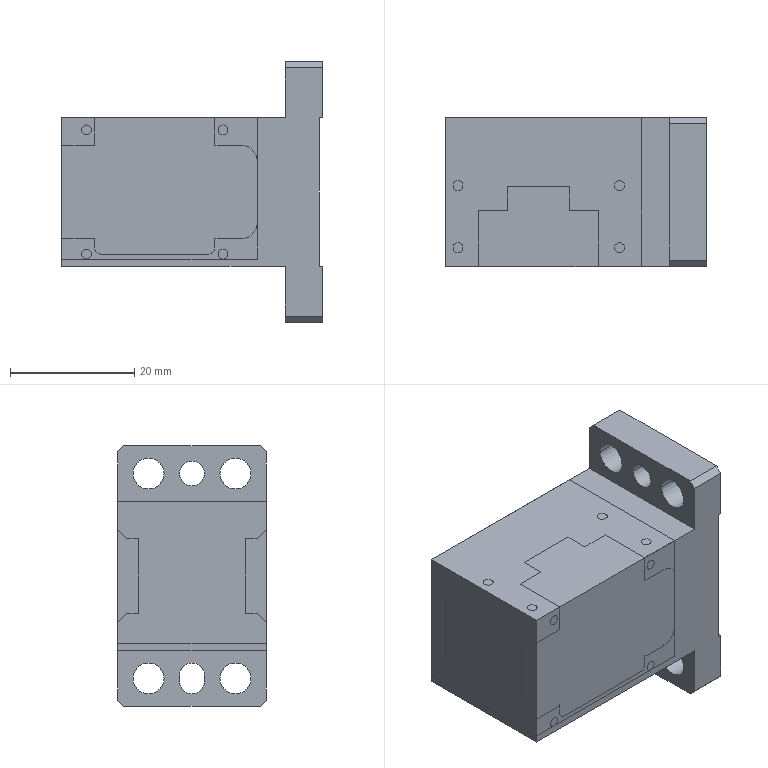NC program | NX | posted with a generic post | part box 42 x 24 x 42 mm
Lines 93 to 952 of 10692:
(ZLEVEL_PROFILE_1 , TOOL : D3)
N172 T03 M6
N174 G54
N176 G17 G0 G90 X-0.064 Y16.054 B0. C0. S6000 M3
N178 G43 Z30. H3
N180 Z0.8
N182 G94 G1 X0.019 Y16.04 Z0.796 F1000.
N184 X0.199 Y16.085 Z0.786
N186 X0.347 Y16.198 Z0.776
N188 X0.44 Y16.364 Z0.766
N190 X0.45 Y16.406 Z0.764
N192 Y16.596 Z0.754
N194 X0.417 Y16.693 Z0.749
N196 X0.303 Y16.846 Z0.739
N198 X0.095 Y16.95 Z0.726
N200 X-0.095 Z0.716
N202 X-0.303 Y16.846 Z0.704
N204 X-0.417 Y16.693 Z0.694
N206 X-0.45 Y16.596 Z0.689
N208 Y16.405 Z0.679
N210 X-0.324 Y16.174 Z0.665
N212 X-0.164 Y16.07 Z0.655
N214 X0.019 Y16.04 Z0.645
N216 X0.199 Y16.085 Z0.636
N218 X0.347 Y16.198 Z0.626
N220 X0.44 Y16.364 Z0.616
N222 X0.45 Y16.406 Z0.614
N224 Y16.596 Z0.604
N226 X0.417 Y16.693 Z0.598
N228 X0.303 Y16.846 Z0.588
N230 X0.095 Y16.95 Z0.576
N232 X-0.095 Z0.566
N234 X-0.303 Y16.846 Z0.554
N236 X-0.417 Y16.693 Z0.544
N238 X-0.45 Y16.596 Z0.539
N240 Y16.405 Z0.529
N242 X-0.324 Y16.174 Z0.515
N244 X-0.164 Y16.07 Z0.505
N246 X0.019 Y16.04 Z0.495
N248 X0.199 Y16.085 Z0.485
N250 X0.347 Y16.198 Z0.476
N252 X0.44 Y16.364 Z0.466
N254 X0.45 Y16.406 Z0.463
N256 Y16.596 Z0.453
N258 X0.417 Y16.693 Z0.448
N260 X0.303 Y16.846 Z0.438
N262 X0.095 Y16.95 Z0.426
N264 X-0.095 Z0.416
N266 X-0.303 Y16.846 Z0.404
N268 X-0.417 Y16.693 Z0.394
N270 X-0.45 Y16.596 Z0.388
N272 Y16.405 Z0.378
N274 X-0.324 Y16.174 Z0.364
N276 X-0.164 Y16.07 Z0.354
N278 X0.019 Y16.04 Z0.345
N280 X0.199 Y16.085 Z0.335
N282 X0.347 Y16.198 Z0.325
N284 X0.44 Y16.364 Z0.315
N286 X0.45 Y16.406 Z0.313
N288 Y16.596 Z0.303
N290 X0.417 Y16.693 Z0.298
N292 X0.303 Y16.846 Z0.288
N294 X0.095 Y16.95 Z0.276
N296 X-0.095 Z0.266
N298 X-0.303 Y16.846 Z0.253
N300 X-0.417 Y16.693 Z0.243
N302 X-0.45 Y16.596 Z0.238
N304 Y16.405 Z0.228
N306 X-0.324 Y16.174 Z0.214
N308 X-0.164 Y16.07 Z0.204
N310 X0.019 Y16.04 Z0.194
N312 X0.199 Y16.085 Z0.185
N314 X0.347 Y16.198 Z0.175
N316 X0.44 Y16.364 Z0.165
N318 X0.45 Y16.406 Z0.163
N320 Y16.596 Z0.153
N322 X0.417 Y16.693 Z0.147
N324 X0.303 Y16.846 Z0.137
N326 X0.095 Y16.95 Z0.125
N328 X-0.095 Z0.115
N330 X-0.303 Y16.846 Z0.103
N332 X-0.417 Y16.693 Z0.093
N334 X-0.45 Y16.596 Z0.088
N336 Y16.405 Z0.078
N338 X-0.324 Y16.174 Z0.064
N340 X-0.164 Y16.07 Z0.054
N342 X0.019 Y16.04 Z0.044
N344 X0.199 Y16.085 Z0.034
N346 X0.347 Y16.198 Z0.025
N348 X0.44 Y16.364 Z0.015
N350 X0.45 Y16.406 Z0.013
N352 Y16.596 Z0.003
N354 X0.417 Y16.693 Z-0.003
N356 X0.303 Y16.846 Z-0.013
N358 X0.095 Y16.95 Z-0.025
N360 X0. Z-0.03
N362 G3 X-0.45 Y16.5 R0.45
N364 X0. Y16.95 R-0.45
N366 G1 X-0.124 Y16.924 Z-0.032
N368 X-0.202 Y16.891 Z-0.034
N370 X-0.274 Y16.845 Z-0.035
N372 X-0.308 Y16.819 Z-0.036
N374 X-0.361 Y16.756 Z-0.038
N376 X-0.403 Y16.681 Z-0.039
N378 X-0.418 Y16.643 Z-0.04
N380 X-0.427 Y16.616
N382 X-0.438 Y16.561 Z-0.041
N384 X-0.441 Y16.475 Z-0.043
N386 X-0.437 Y16.433 Z-0.044
N388 X-0.432 Y16.406
N390 X-0.417 Y16.353 Z-0.045
N392 X-0.38 Y16.275 Z-0.047
N394 X-0.357 Y16.24
N396 X-0.341 Y16.218 Z-0.048
N398 X-0.303 Y16.178 Z-0.049
N400 X-0.234 Y16.126 Z-0.05
N402 X-0.198 Y16.105 Z-0.051
N404 X-0.173 Y16.093 Z-0.052
N406 X-0.121 Y16.075 Z-0.053
N408 X-0.039 Y16.06 Z-0.054
N410 X0.002 Y16.056 Z-0.055
N412 X0.088 Y16.066 Z-0.056
N414 X0.188 Y16.101 Z-0.058
N416 X0.282 Y16.149 Z-0.06
N418 G3 X0. Y16.95 R0.45
N420 G1 X-0.124 Y16.924 Z-0.062
N422 X-0.202 Y16.891 Z-0.064
N424 X-0.274 Y16.845 Z-0.065
N426 X-0.308 Y16.819 Z-0.066
N428 X-0.361 Y16.756 Z-0.068
N430 X-0.403 Y16.681 Z-0.069
N432 X-0.418 Y16.643 Z-0.07
N434 X-0.427 Y16.616
N436 X-0.438 Y16.561 Z-0.071
N438 X-0.441 Y16.475 Z-0.073
N440 X-0.437 Y16.433 Z-0.074
N442 X-0.432 Y16.406
N444 X-0.417 Y16.353 Z-0.075
N446 X-0.38 Y16.275 Z-0.077
N448 X-0.357 Y16.24
N450 X-0.341 Y16.218 Z-0.078
N452 X-0.303 Y16.178 Z-0.079
N454 X-0.234 Y16.126 Z-0.08
N456 X-0.198 Y16.105 Z-0.081
N458 X-0.173 Y16.093 Z-0.082
N460 X-0.121 Y16.075 Z-0.083
N462 X-0.039 Y16.06 Z-0.084
N464 X0.002 Y16.056 Z-0.085
N466 X0.088 Y16.066 Z-0.086
N468 X0.188 Y16.101 Z-0.088
N470 X0.282 Y16.149 Z-0.09
N472 G3 X0. Y16.95 R0.45
N474 G1 X-0.124 Y16.924 Z-0.092
N476 X-0.202 Y16.891 Z-0.094
N478 X-0.274 Y16.845 Z-0.095
N480 X-0.308 Y16.819 Z-0.096
N482 X-0.361 Y16.756 Z-0.098
N484 X-0.403 Y16.681 Z-0.099
N486 X-0.418 Y16.643 Z-0.1
N488 X-0.427 Y16.616
N490 X-0.438 Y16.561 Z-0.101
N492 X-0.441 Y16.475 Z-0.103
N494 X-0.437 Y16.433 Z-0.104
N496 X-0.432 Y16.406
N498 X-0.417 Y16.353 Z-0.105
N500 X-0.38 Y16.275 Z-0.107
N502 X-0.357 Y16.24
N504 X-0.341 Y16.218 Z-0.108
N506 X-0.303 Y16.178 Z-0.109
N508 X-0.234 Y16.126 Z-0.11
N510 X-0.198 Y16.105 Z-0.111
N512 X-0.173 Y16.093 Z-0.112
N514 X-0.121 Y16.075 Z-0.113
N516 X-0.039 Y16.06 Z-0.114
N518 X0.002 Y16.056 Z-0.115
N520 X0.088 Y16.066 Z-0.116
N522 X0.188 Y16.101 Z-0.118
N524 X0.282 Y16.149 Z-0.12
N526 G3 X0. Y16.95 R0.45
N528 G1 X-0.124 Y16.924 Z-0.122
N530 X-0.202 Y16.891 Z-0.124
N532 X-0.274 Y16.845 Z-0.125
N534 X-0.308 Y16.819 Z-0.126
N536 X-0.361 Y16.756 Z-0.128
N538 X-0.403 Y16.681 Z-0.129
N540 X-0.418 Y16.643 Z-0.13
N542 X-0.427 Y16.616
N544 X-0.438 Y16.561 Z-0.131
N546 X-0.441 Y16.475 Z-0.133
N548 X-0.437 Y16.433 Z-0.134
N550 X-0.432 Y16.406
N552 X-0.417 Y16.353 Z-0.135
N554 X-0.38 Y16.275 Z-0.137
N556 X-0.357 Y16.24
N558 X-0.341 Y16.218 Z-0.138
N560 X-0.303 Y16.178 Z-0.139
N562 X-0.234 Y16.126 Z-0.14
N564 X-0.198 Y16.105 Z-0.141
N566 X-0.173 Y16.093 Z-0.142
N568 X-0.121 Y16.075 Z-0.143
N570 X-0.039 Y16.06 Z-0.144
N572 X0.002 Y16.056 Z-0.145
N574 X0.088 Y16.066 Z-0.146
N576 X0.188 Y16.101 Z-0.148
N578 X0.282 Y16.149 Z-0.15
N580 G3 X0. Y16.95 R0.45
N582 G1 X-0.124 Y16.924 Z-0.152
N584 X-0.202 Y16.891 Z-0.154
N586 X-0.274 Y16.845 Z-0.155
N588 X-0.308 Y16.819 Z-0.156
N590 X-0.361 Y16.756 Z-0.158
N592 X-0.403 Y16.681 Z-0.159
N594 X-0.418 Y16.643 Z-0.16
N596 X-0.427 Y16.616
N598 X-0.438 Y16.561 Z-0.161
N600 X-0.441 Y16.475 Z-0.163
N602 X-0.437 Y16.433 Z-0.164
N604 X-0.432 Y16.406
N606 X-0.417 Y16.353 Z-0.165
N608 X-0.38 Y16.275 Z-0.167
N610 X-0.357 Y16.24
N612 X-0.341 Y16.218 Z-0.168
N614 X-0.303 Y16.178 Z-0.169
N616 X-0.234 Y16.126 Z-0.17
N618 X-0.198 Y16.105 Z-0.171
N620 X-0.173 Y16.093 Z-0.172
N622 X-0.121 Y16.075 Z-0.173
N624 X-0.039 Y16.06 Z-0.174
N626 X0.002 Y16.056 Z-0.175
N628 X0.088 Y16.066 Z-0.176
N630 X0.188 Y16.101 Z-0.178
N632 X0.282 Y16.149 Z-0.18
N634 G3 X0. Y16.95 R0.45
N636 G1 X-0.124 Y16.924 Z-0.182
N638 X-0.202 Y16.891 Z-0.184
N640 X-0.274 Y16.845 Z-0.185
N642 X-0.308 Y16.819 Z-0.186
N644 X-0.361 Y16.756 Z-0.188
N646 X-0.403 Y16.681 Z-0.189
N648 X-0.418 Y16.643 Z-0.19
N650 X-0.427 Y16.616
N652 X-0.438 Y16.561 Z-0.191
N654 X-0.441 Y16.475 Z-0.193
N656 X-0.437 Y16.433 Z-0.194
N658 X-0.432 Y16.406
N660 X-0.417 Y16.353 Z-0.195
N662 X-0.38 Y16.275 Z-0.197
N664 X-0.357 Y16.24
N666 X-0.341 Y16.218 Z-0.198
N668 X-0.303 Y16.178 Z-0.199
N670 X-0.234 Y16.126 Z-0.2
N672 X-0.198 Y16.105 Z-0.201
N674 X-0.173 Y16.093 Z-0.202
N676 X-0.121 Y16.075 Z-0.203
N678 X-0.039 Y16.06 Z-0.204
N680 X0.002 Y16.056 Z-0.205
N682 X0.088 Y16.066 Z-0.206
N684 X0.188 Y16.101 Z-0.208
N686 X0.282 Y16.149 Z-0.21
N688 G3 X0. Y16.95 R0.45
N690 G1 X-0.124 Y16.924 Z-0.212
N692 X-0.202 Y16.891 Z-0.214
N694 X-0.274 Y16.845 Z-0.215
N696 X-0.308 Y16.819 Z-0.216
N698 X-0.361 Y16.756 Z-0.218
N700 X-0.403 Y16.681 Z-0.219
N702 X-0.418 Y16.643 Z-0.22
N704 X-0.427 Y16.616
N706 X-0.438 Y16.561 Z-0.221
N708 X-0.441 Y16.475 Z-0.223
N710 X-0.437 Y16.433 Z-0.224
N712 X-0.432 Y16.406
N714 X-0.417 Y16.353 Z-0.225
N716 X-0.38 Y16.275 Z-0.227
N718 X-0.357 Y16.24
N720 X-0.341 Y16.218 Z-0.228
N722 X-0.303 Y16.178 Z-0.229
N724 X-0.234 Y16.126 Z-0.23
N726 X-0.198 Y16.105 Z-0.231
N728 X-0.173 Y16.093 Z-0.232
N730 X-0.121 Y16.075 Z-0.233
N732 X-0.039 Y16.06 Z-0.234
N734 X0.002 Y16.056 Z-0.235
N736 X0.088 Y16.066 Z-0.236
N738 X0.188 Y16.101 Z-0.238
N740 X0.282 Y16.149 Z-0.24
N742 G3 X0. Y16.95 R0.45
N744 G1 X-0.124 Y16.924 Z-0.242
N746 X-0.202 Y16.891 Z-0.244
N748 X-0.274 Y16.845 Z-0.245
N750 X-0.308 Y16.819 Z-0.246
N752 X-0.361 Y16.756 Z-0.248
N754 X-0.403 Y16.681 Z-0.249
N756 X-0.418 Y16.643 Z-0.25
N758 X-0.427 Y16.616
N760 X-0.438 Y16.561 Z-0.251
N762 X-0.441 Y16.475 Z-0.253
N764 X-0.437 Y16.433 Z-0.254
N766 X-0.432 Y16.406
N768 X-0.417 Y16.353 Z-0.255
N770 X-0.38 Y16.275 Z-0.257
N772 X-0.357 Y16.24
N774 X-0.341 Y16.218 Z-0.258
N776 X-0.303 Y16.178 Z-0.259
N778 X-0.234 Y16.126 Z-0.26
N780 X-0.198 Y16.105 Z-0.261
N782 X-0.173 Y16.093 Z-0.262
N784 X-0.121 Y16.075 Z-0.263
N786 X-0.039 Y16.06 Z-0.264
N788 X0.002 Y16.056 Z-0.265
N790 X0.088 Y16.066 Z-0.266
N792 X0.188 Y16.101 Z-0.268
N794 X0.282 Y16.149 Z-0.27
N796 G3 X0. Y16.95 R0.45
N798 G1 X-0.124 Y16.924 Z-0.272
N800 X-0.202 Y16.891 Z-0.274
N802 X-0.274 Y16.845 Z-0.275
N804 X-0.308 Y16.819 Z-0.276
N806 X-0.361 Y16.756 Z-0.278
N808 X-0.403 Y16.681 Z-0.279
N810 X-0.418 Y16.643 Z-0.28
N812 X-0.427 Y16.616
N814 X-0.438 Y16.561 Z-0.281
N816 X-0.441 Y16.475 Z-0.283
N818 X-0.437 Y16.433 Z-0.284
N820 X-0.432 Y16.406
N822 X-0.417 Y16.353 Z-0.285
N824 X-0.38 Y16.275 Z-0.287
N826 X-0.357 Y16.24
N828 X-0.341 Y16.218 Z-0.288
N830 X-0.303 Y16.178 Z-0.289
N832 X-0.234 Y16.126 Z-0.29
N834 X-0.198 Y16.105 Z-0.291
N836 X-0.173 Y16.093 Z-0.292
N838 X-0.121 Y16.075 Z-0.293
N840 X-0.039 Y16.06 Z-0.294
N842 X0.002 Y16.056 Z-0.295
N844 X0.088 Y16.066 Z-0.296
N846 X0.188 Y16.101 Z-0.298
N848 X0.282 Y16.149 Z-0.3
N850 G3 X0. Y16.95 R0.45
N852 G1 X-0.124 Y16.924 Z-0.302
N854 X-0.202 Y16.891 Z-0.304
N856 X-0.274 Y16.845 Z-0.305
N858 X-0.308 Y16.819 Z-0.306
N860 X-0.361 Y16.756 Z-0.308
N862 X-0.403 Y16.681 Z-0.309
N864 X-0.418 Y16.643 Z-0.31
N866 X-0.427 Y16.616
N868 X-0.438 Y16.561 Z-0.311
N870 X-0.441 Y16.475 Z-0.313
N872 X-0.437 Y16.433 Z-0.314
N874 X-0.432 Y16.406
N876 X-0.417 Y16.353 Z-0.315
N878 X-0.38 Y16.275 Z-0.317
N880 X-0.357 Y16.24
N882 X-0.341 Y16.218 Z-0.318
N884 X-0.303 Y16.178 Z-0.319
N886 X-0.234 Y16.126 Z-0.32
N888 X-0.198 Y16.105 Z-0.321
N890 X-0.173 Y16.093 Z-0.322
N892 X-0.121 Y16.075 Z-0.323
N894 X-0.039 Y16.06 Z-0.324
N896 X0.002 Y16.056 Z-0.325
N898 X0.088 Y16.066 Z-0.326
N900 X0.188 Y16.101 Z-0.328
N902 X0.282 Y16.149 Z-0.33
N904 G3 X0. Y16.95 R0.45
N906 G1 X-0.124 Y16.924 Z-0.332
N908 X-0.202 Y16.891 Z-0.334
N910 X-0.274 Y16.845 Z-0.335
N912 X-0.308 Y16.819 Z-0.336
N914 X-0.361 Y16.756 Z-0.338
N916 X-0.403 Y16.681 Z-0.339
N918 X-0.418 Y16.643 Z-0.34
N920 X-0.427 Y16.616
N922 X-0.438 Y16.561 Z-0.341
N924 X-0.441 Y16.475 Z-0.343
N926 X-0.437 Y16.433 Z-0.344
N928 X-0.432 Y16.406
N930 X-0.417 Y16.353 Z-0.345
N932 X-0.38 Y16.275 Z-0.347
N934 X-0.357 Y16.24
N936 X-0.341 Y16.218 Z-0.348
N938 X-0.303 Y16.178 Z-0.349
N940 X-0.234 Y16.126 Z-0.35
N942 X-0.198 Y16.105 Z-0.351
N944 X-0.173 Y16.093 Z-0.352
N946 X-0.121 Y16.075 Z-0.353
N948 X-0.039 Y16.06 Z-0.354
N950 X0.002 Y16.056 Z-0.355
N952 X0.088 Y16.066 Z-0.356
N954 X0.188 Y16.101 Z-0.358
N956 X0.282 Y16.149 Z-0.36
N958 G3 X0. Y16.95 R0.45
N960 G1 X-0.124 Y16.924 Z-0.362
N962 X-0.202 Y16.891 Z-0.364
N964 X-0.274 Y16.845 Z-0.365
N966 X-0.308 Y16.819 Z-0.366
N968 X-0.361 Y16.756 Z-0.368
N970 X-0.403 Y16.681 Z-0.369
N972 X-0.418 Y16.643 Z-0.37
N974 X-0.427 Y16.616
N976 X-0.438 Y16.561 Z-0.371
N978 X-0.441 Y16.475 Z-0.373
N980 X-0.437 Y16.433 Z-0.374
N982 X-0.432 Y16.406
N984 X-0.417 Y16.353 Z-0.375
N986 X-0.38 Y16.275 Z-0.377
N988 X-0.357 Y16.24
N990 X-0.341 Y16.218 Z-0.378
N992 X-0.303 Y16.178 Z-0.379
N994 X-0.234 Y16.126 Z-0.38
N996 X-0.198 Y16.105 Z-0.381
N998 X-0.173 Y16.093 Z-0.382
N1000 X-0.121 Y16.075 Z-0.383
N1002 X-0.039 Y16.06 Z-0.384
N1004 X0.002 Y16.056 Z-0.385
N1006 X0.088 Y16.066 Z-0.386
N1008 X0.188 Y16.101 Z-0.388
N1010 X0.282 Y16.149 Z-0.39
N1012 G3 X0. Y16.95 R0.45
N1014 G1 X-0.124 Y16.924 Z-0.392
N1016 X-0.202 Y16.891 Z-0.394
N1018 X-0.274 Y16.845 Z-0.395
N1020 X-0.308 Y16.819 Z-0.396
N1022 X-0.361 Y16.756 Z-0.398
N1024 X-0.403 Y16.681 Z-0.399
N1026 X-0.418 Y16.643 Z-0.4
N1028 X-0.427 Y16.616
N1030 X-0.438 Y16.561 Z-0.401
N1032 X-0.441 Y16.475 Z-0.403
N1034 X-0.437 Y16.433 Z-0.404
N1036 X-0.432 Y16.406
N1038 X-0.417 Y16.353 Z-0.405
N1040 X-0.38 Y16.275 Z-0.407
N1042 X-0.357 Y16.24
N1044 X-0.341 Y16.218 Z-0.408
N1046 X-0.303 Y16.178 Z-0.409
N1048 X-0.234 Y16.126 Z-0.41
N1050 X-0.198 Y16.105 Z-0.411
N1052 X-0.173 Y16.093 Z-0.412
N1054 X-0.121 Y16.075 Z-0.413
N1056 X-0.039 Y16.06 Z-0.414
N1058 X0.002 Y16.056 Z-0.415
N1060 X0.088 Y16.066 Z-0.416
N1062 X0.188 Y16.101 Z-0.418
N1064 X0.282 Y16.149 Z-0.42
N1066 G3 X0. Y16.95 R0.45
N1068 G1 X-0.124 Y16.924 Z-0.422
N1070 X-0.202 Y16.891 Z-0.424
N1072 X-0.274 Y16.845 Z-0.425
N1074 X-0.308 Y16.819 Z-0.426
N1076 X-0.361 Y16.756 Z-0.428
N1078 X-0.403 Y16.681 Z-0.429
N1080 X-0.418 Y16.643 Z-0.43
N1082 X-0.427 Y16.616
N1084 X-0.438 Y16.561 Z-0.431
N1086 X-0.441 Y16.475 Z-0.433
N1088 X-0.437 Y16.434 Z-0.434
N1090 X-0.432 Y16.406
N1092 X-0.417 Y16.353 Z-0.435
N1094 X-0.38 Y16.275 Z-0.437
N1096 X-0.357 Y16.24
N1098 X-0.341 Y16.218 Z-0.438
N1100 X-0.303 Y16.178 Z-0.439
N1102 X-0.234 Y16.126 Z-0.44
N1104 X-0.198 Y16.105 Z-0.441
N1106 X-0.173 Y16.093 Z-0.442
N1108 X-0.121 Y16.075 Z-0.443
N1110 X-0.039 Y16.06 Z-0.444
N1112 X0.002 Y16.056 Z-0.445
N1114 X0.088 Y16.066 Z-0.446
N1116 X0.188 Y16.101 Z-0.448
N1118 X0.282 Y16.149 Z-0.45
N1120 G3 X0. Y16.95 R0.45
N1122 G1 X-0.124 Y16.924 Z-0.452
N1124 X-0.202 Y16.891 Z-0.454
N1126 X-0.274 Y16.845 Z-0.455
N1128 X-0.308 Y16.819 Z-0.456
N1130 X-0.361 Y16.756 Z-0.458
N1132 X-0.403 Y16.681 Z-0.459
N1134 X-0.418 Y16.643 Z-0.46
N1136 X-0.427 Y16.616
N1138 X-0.438 Y16.561 Z-0.461
N1140 X-0.441 Y16.475 Z-0.463
N1142 X-0.437 Y16.434 Z-0.464
N1144 X-0.432 Y16.406
N1146 X-0.417 Y16.353 Z-0.465
N1148 X-0.38 Y16.275 Z-0.467
N1150 X-0.357 Y16.24
N1152 X-0.341 Y16.218 Z-0.468
N1154 X-0.303 Y16.178 Z-0.469
N1156 X-0.234 Y16.126 Z-0.47
N1158 X-0.198 Y16.105 Z-0.471
N1160 X-0.173 Y16.093 Z-0.472
N1162 X-0.121 Y16.075 Z-0.473
N1164 X-0.039 Y16.06 Z-0.474
N1166 X0.002 Y16.056 Z-0.475
N1168 X0.088 Y16.066 Z-0.476
N1170 X0.188 Y16.101 Z-0.478
N1172 X0.282 Y16.149 Z-0.48
N1174 G3 X0. Y16.95 R0.45
N1176 G1 X-0.124 Y16.924 Z-0.482
N1178 X-0.202 Y16.891 Z-0.484
N1180 X-0.274 Y16.845 Z-0.485
N1182 X-0.308 Y16.819 Z-0.486
N1184 X-0.361 Y16.756 Z-0.488
N1186 X-0.403 Y16.681 Z-0.489
N1188 X-0.418 Y16.643 Z-0.49
N1190 X-0.427 Y16.616
N1192 X-0.438 Y16.561 Z-0.491
N1194 X-0.441 Y16.475 Z-0.493
N1196 X-0.437 Y16.434 Z-0.494
N1198 X-0.432 Y16.406
N1200 X-0.417 Y16.353 Z-0.495
N1202 X-0.38 Y16.275 Z-0.497
N1204 X-0.357 Y16.24
N1206 X-0.341 Y16.218 Z-0.498
N1208 X-0.303 Y16.178 Z-0.499
N1210 X-0.234 Y16.126 Z-0.5
N1212 X-0.198 Y16.105 Z-0.501
N1214 X-0.173 Y16.093 Z-0.502
N1216 X-0.121 Y16.075 Z-0.503
N1218 X-0.039 Y16.06 Z-0.504
N1220 X0.002 Y16.056 Z-0.505
N1222 X0.088 Y16.066 Z-0.506
N1224 X0.188 Y16.101 Z-0.508
N1226 X0.282 Y16.149 Z-0.51
N1228 G3 X0. Y16.95 R0.45
N1230 G1 X-0.124 Y16.924 Z-0.512
N1232 X-0.202 Y16.891 Z-0.514
N1234 X-0.274 Y16.845 Z-0.515
N1236 X-0.308 Y16.819 Z-0.516
N1238 X-0.361 Y16.756 Z-0.518
N1240 X-0.403 Y16.681 Z-0.519
N1242 X-0.418 Y16.643 Z-0.52
N1244 X-0.427 Y16.616
N1246 X-0.438 Y16.561 Z-0.521
N1248 X-0.441 Y16.475 Z-0.523
N1250 X-0.437 Y16.434 Z-0.524
N1252 X-0.432 Y16.406
N1254 X-0.417 Y16.353 Z-0.525
N1256 X-0.38 Y16.275 Z-0.527
N1258 X-0.357 Y16.24
N1260 X-0.341 Y16.218 Z-0.528
N1262 X-0.303 Y16.178 Z-0.529
N1264 X-0.234 Y16.126 Z-0.53
N1266 X-0.198 Y16.105 Z-0.531
N1268 X-0.173 Y16.093 Z-0.532
N1270 X-0.121 Y16.075 Z-0.533
N1272 X-0.039 Y16.06 Z-0.534
N1274 X0.002 Y16.056 Z-0.535
N1276 X0.088 Y16.066 Z-0.536
N1278 X0.188 Y16.101 Z-0.538
N1280 X0.282 Y16.149 Z-0.54
N1282 G3 X0. Y16.95 R0.45
N1284 G1 X-0.124 Y16.924 Z-0.542
N1286 X-0.202 Y16.891 Z-0.544
N1288 X-0.274 Y16.845 Z-0.545
N1290 X-0.308 Y16.819 Z-0.546
N1292 X-0.361 Y16.756 Z-0.548
N1294 X-0.403 Y16.681 Z-0.549
N1296 X-0.418 Y16.643 Z-0.55
N1298 X-0.427 Y16.616
N1300 X-0.438 Y16.561 Z-0.551
N1302 X-0.441 Y16.475 Z-0.553
N1304 X-0.437 Y16.434 Z-0.554
N1306 X-0.432 Y16.406
N1308 X-0.417 Y16.353 Z-0.555
N1310 X-0.38 Y16.275 Z-0.557
N1312 X-0.357 Y16.24
N1314 X-0.341 Y16.218 Z-0.558
N1316 X-0.303 Y16.178 Z-0.559
N1318 X-0.234 Y16.126 Z-0.56
N1320 X-0.198 Y16.105 Z-0.561
N1322 X-0.173 Y16.093 Z-0.562
N1324 X-0.121 Y16.075 Z-0.563
N1326 X-0.039 Y16.06 Z-0.564
N1328 X0.002 Y16.056 Z-0.565
N1330 X0.088 Y16.066 Z-0.566
N1332 X0.188 Y16.101 Z-0.568
N1334 X0.282 Y16.149 Z-0.57
N1336 G3 X0. Y16.95 R0.45
N1338 G1 X-0.124 Y16.924 Z-0.572
N1340 X-0.202 Y16.891 Z-0.574
N1342 X-0.274 Y16.845 Z-0.575
N1344 X-0.308 Y16.819 Z-0.576
N1346 X-0.361 Y16.756 Z-0.578
N1348 X-0.403 Y16.681 Z-0.579
N1350 X-0.418 Y16.643 Z-0.58
N1352 X-0.427 Y16.616
N1354 X-0.438 Y16.561 Z-0.581
N1356 X-0.441 Y16.475 Z-0.583
N1358 X-0.437 Y16.434 Z-0.584
N1360 X-0.432 Y16.406
N1362 X-0.417 Y16.353 Z-0.585
N1364 X-0.38 Y16.275 Z-0.587
N1366 X-0.357 Y16.24
N1368 X-0.341 Y16.218 Z-0.588
N1370 X-0.303 Y16.178 Z-0.589
N1372 X-0.234 Y16.126 Z-0.59
N1374 X-0.198 Y16.105 Z-0.591
N1376 X-0.173 Y16.093 Z-0.592
N1378 X-0.121 Y16.075 Z-0.593
N1380 X-0.039 Y16.06 Z-0.594
N1382 X0.002 Y16.056 Z-0.595
N1384 X0.088 Y16.066 Z-0.596
N1386 X0.188 Y16.101 Z-0.598
N1388 X0.282 Y16.149 Z-0.6
N1390 G3 X0. Y16.95 R0.45
N1392 G1 X-0.124 Y16.924 Z-0.602
N1394 X-0.202 Y16.891 Z-0.604
N1396 X-0.274 Y16.845 Z-0.605
N1398 X-0.308 Y16.819 Z-0.606
N1400 X-0.361 Y16.756 Z-0.608
N1402 X-0.403 Y16.681 Z-0.609
N1404 X-0.418 Y16.643 Z-0.61
N1406 X-0.427 Y16.616
N1408 X-0.438 Y16.561 Z-0.611
N1410 X-0.441 Y16.475 Z-0.613
N1412 X-0.437 Y16.434 Z-0.614
N1414 X-0.432 Y16.406
N1416 X-0.417 Y16.353 Z-0.615
N1418 X-0.38 Y16.275 Z-0.617
N1420 X-0.357 Y16.24
N1422 X-0.341 Y16.218 Z-0.618
N1424 X-0.303 Y16.178 Z-0.619
N1426 X-0.234 Y16.126 Z-0.62
N1428 X-0.198 Y16.105 Z-0.621
N1430 X-0.173 Y16.093 Z-0.622
N1432 X-0.121 Y16.075 Z-0.623
N1434 X-0.039 Y16.06 Z-0.624
N1436 X0.002 Y16.056 Z-0.625
N1438 X0.088 Y16.066 Z-0.626
N1440 X0.188 Y16.101 Z-0.628
N1442 X0.282 Y16.149 Z-0.63
N1444 G3 X0. Y16.95 R0.45
N1446 G1 X-0.124 Y16.924 Z-0.632
N1448 X-0.202 Y16.891 Z-0.634
N1450 X-0.274 Y16.845 Z-0.635
N1452 X-0.308 Y16.819 Z-0.636
N1454 X-0.361 Y16.756 Z-0.638
N1456 X-0.403 Y16.681 Z-0.639
N1458 X-0.418 Y16.643 Z-0.64
N1460 X-0.427 Y16.616
N1462 X-0.438 Y16.561 Z-0.641
N1464 X-0.441 Y16.475 Z-0.643
N1466 X-0.437 Y16.434 Z-0.644
N1468 X-0.432 Y16.406
N1470 X-0.417 Y16.353 Z-0.645
N1472 X-0.38 Y16.275 Z-0.647
N1474 X-0.357 Y16.24
N1476 X-0.341 Y16.218 Z-0.648
N1478 X-0.303 Y16.178 Z-0.649
N1480 X-0.234 Y16.126 Z-0.65
N1482 X-0.198 Y16.105 Z-0.651
N1484 X-0.173 Y16.093 Z-0.652
N1486 X-0.121 Y16.075 Z-0.653
N1488 X-0.039 Y16.06 Z-0.654
N1490 X0.002 Y16.056 Z-0.655
N1492 X0.088 Y16.066 Z-0.656
N1494 X0.188 Y16.101 Z-0.658
N1496 X0.282 Y16.149 Z-0.66
N1498 G3 X0. Y16.95 R0.45
N1500 G1 X-0.124 Y16.924 Z-0.662
N1502 X-0.202 Y16.891 Z-0.664
N1504 X-0.274 Y16.845 Z-0.665
N1506 X-0.308 Y16.819 Z-0.666
N1508 X-0.361 Y16.756 Z-0.668
N1510 X-0.403 Y16.681 Z-0.669
N1512 X-0.418 Y16.643 Z-0.67
N1514 X-0.427 Y16.616
N1516 X-0.438 Y16.561 Z-0.671
N1518 X-0.441 Y16.475 Z-0.673
N1520 X-0.437 Y16.434 Z-0.674
N1522 X-0.432 Y16.406
N1524 X-0.417 Y16.353 Z-0.675
N1526 X-0.38 Y16.275 Z-0.677
N1528 X-0.357 Y16.24
N1530 X-0.341 Y16.218 Z-0.678
N1532 X-0.303 Y16.178 Z-0.679
N1534 X-0.234 Y16.126 Z-0.68
N1536 X-0.198 Y16.105 Z-0.681
N1538 X-0.173 Y16.093 Z-0.682
N1540 X-0.121 Y16.075 Z-0.683
N1542 X-0.039 Y16.06 Z-0.684
N1544 X0.002 Y16.056 Z-0.685
N1546 X0.088 Y16.066 Z-0.686
N1548 X0.188 Y16.101 Z-0.688
N1550 X0.282 Y16.149 Z-0.69
N1552 G3 X0. Y16.95 R0.45
N1554 G1 X-0.124 Y16.924 Z-0.692
N1556 X-0.202 Y16.891 Z-0.694
N1558 X-0.274 Y16.845 Z-0.695
N1560 X-0.308 Y16.819 Z-0.696
N1562 X-0.361 Y16.756 Z-0.698
N1564 X-0.403 Y16.681 Z-0.699
N1566 X-0.418 Y16.643 Z-0.7
N1568 X-0.427 Y16.616
N1570 X-0.438 Y16.561 Z-0.701
N1572 X-0.441 Y16.475 Z-0.703
N1574 X-0.437 Y16.434 Z-0.704
N1576 X-0.432 Y16.406
N1578 X-0.417 Y16.353 Z-0.705
N1580 X-0.38 Y16.275 Z-0.707
N1582 X-0.357 Y16.24
N1584 X-0.341 Y16.218 Z-0.708
N1586 X-0.303 Y16.178 Z-0.709
N1588 X-0.234 Y16.126 Z-0.71
N1590 X-0.198 Y16.105 Z-0.711
N1592 X-0.173 Y16.093 Z-0.712
N1594 X-0.121 Y16.075 Z-0.713
N1596 X-0.039 Y16.06 Z-0.714
N1598 X0.002 Y16.056 Z-0.715
N1600 X0.088 Y16.066 Z-0.716
N1602 X0.188 Y16.101 Z-0.718
N1604 X0.282 Y16.149 Z-0.72
N1606 G3 X0. Y16.95 R0.45
N1608 G1 X-0.124 Y16.924 Z-0.722
N1610 X-0.202 Y16.891 Z-0.724
N1612 X-0.274 Y16.845 Z-0.725
N1614 X-0.308 Y16.819 Z-0.726
N1616 X-0.361 Y16.756 Z-0.728
N1618 X-0.403 Y16.681 Z-0.729
N1620 X-0.418 Y16.643 Z-0.73
N1622 X-0.427 Y16.616
N1624 X-0.438 Y16.561 Z-0.731
N1626 X-0.441 Y16.475 Z-0.733
N1628 X-0.437 Y16.434 Z-0.734
N1630 X-0.432 Y16.406
N1632 X-0.417 Y16.353 Z-0.735
N1634 X-0.38 Y16.275 Z-0.737
N1636 X-0.357 Y16.24
N1638 X-0.341 Y16.218 Z-0.738
N1640 X-0.303 Y16.178 Z-0.739
N1642 X-0.234 Y16.126 Z-0.74
N1644 X-0.198 Y16.105 Z-0.741
N1646 X-0.173 Y16.093 Z-0.742
N1648 X-0.121 Y16.075 Z-0.743
N1650 X-0.039 Y16.06 Z-0.744
N1652 X0.002 Y16.056 Z-0.745
N1654 X0.088 Y16.066 Z-0.746
N1656 X0.188 Y16.101 Z-0.748
N1658 X0.282 Y16.149 Z-0.75
N1660 G3 X0. Y16.95 R0.45
N1662 G1 X-0.124 Y16.924 Z-0.752
N1664 X-0.202 Y16.891 Z-0.754
N1666 X-0.274 Y16.845 Z-0.755
N1668 X-0.308 Y16.819 Z-0.756
N1670 X-0.361 Y16.756 Z-0.758
N1672 X-0.403 Y16.681 Z-0.759
N1674 X-0.418 Y16.643 Z-0.76
N1676 X-0.427 Y16.616
N1678 X-0.438 Y16.561 Z-0.761
N1680 X-0.441 Y16.475 Z-0.763
N1682 X-0.437 Y16.434 Z-0.764
N1684 X-0.432 Y16.406
N1686 X-0.417 Y16.353 Z-0.765
N1688 X-0.38 Y16.275 Z-0.767
N1690 X-0.357 Y16.24
N1692 X-0.341 Y16.218 Z-0.768
N1694 X-0.303 Y16.178 Z-0.769
N1696 X-0.234 Y16.126 Z-0.77
N1698 X-0.198 Y16.105 Z-0.771
N1700 X-0.173 Y16.093 Z-0.772
N1702 X-0.121 Y16.075 Z-0.773
N1704 X-0.039 Y16.06 Z-0.774
N1706 X0.002 Y16.056 Z-0.775
N1708 X0.088 Y16.066 Z-0.776
N1710 X0.188 Y16.101 Z-0.778
N1712 X0.282 Y16.149 Z-0.78
N1714 G3 X0. Y16.95 R0.45
N1716 G1 X-0.124 Y16.924 Z-0.782
N1718 X-0.202 Y16.891 Z-0.784
N1720 X-0.274 Y16.845 Z-0.785
N1722 X-0.308 Y16.819 Z-0.786
N1724 X-0.361 Y16.756 Z-0.788
N1726 X-0.403 Y16.681 Z-0.789
N1728 X-0.418 Y16.643 Z-0.79
N1730 X-0.427 Y16.616
N1732 X-0.438 Y16.561 Z-0.791
N1734 X-0.441 Y16.475 Z-0.793
N1736 X-0.437 Y16.434 Z-0.794
N1738 X-0.432 Y16.406
N1740 X-0.417 Y16.353 Z-0.795
N1742 X-0.38 Y16.275 Z-0.797
N1744 X-0.357 Y16.24
N1746 X-0.341 Y16.218 Z-0.798
N1748 X-0.303 Y16.178 Z-0.799
N1750 X-0.234 Y16.126 Z-0.8
N1752 X-0.198 Y16.105 Z-0.801
N1754 X-0.173 Y16.093 Z-0.802
N1756 X-0.121 Y16.075 Z-0.803
N1758 X-0.039 Y16.06 Z-0.804
N1760 X0.002 Y16.056 Z-0.805
N1762 X0.088 Y16.066 Z-0.806
N1764 X0.188 Y16.101 Z-0.808
N1766 X0.282 Y16.149 Z-0.81
N1768 G3 X0. Y16.95 R0.45
N1770 G1 X-0.124 Y16.924 Z-0.812
N1772 X-0.202 Y16.891 Z-0.814
N1774 X-0.274 Y16.845 Z-0.815
N1776 X-0.308 Y16.819 Z-0.816
N1778 X-0.361 Y16.756 Z-0.818
N1780 X-0.403 Y16.681 Z-0.819
N1782 X-0.418 Y16.643 Z-0.82
N1784 X-0.427 Y16.616
N1786 X-0.438 Y16.561 Z-0.821
N1788 X-0.441 Y16.475 Z-0.823
N1790 X-0.437 Y16.434 Z-0.824
N1792 X-0.432 Y16.406
N1794 X-0.417 Y16.353 Z-0.825
N1796 X-0.38 Y16.275 Z-0.827
N1798 X-0.357 Y16.24
N1800 X-0.341 Y16.218 Z-0.828
N1802 X-0.303 Y16.178 Z-0.829
N1804 X-0.234 Y16.126 Z-0.83
N1806 X-0.198 Y16.105 Z-0.831
N1808 X-0.173 Y16.093 Z-0.832
N1810 X-0.121 Y16.075 Z-0.833
N1812 X-0.039 Y16.06 Z-0.834
N1814 X0.002 Y16.056 Z-0.835
N1816 X0.088 Y16.066 Z-0.836
N1818 X0.188 Y16.101 Z-0.838
N1820 X0.282 Y16.149 Z-0.84
N1822 G3 X0. Y16.95 R0.45
N1824 G1 X-0.124 Y16.924 Z-0.842
N1826 X-0.202 Y16.891 Z-0.844
N1828 X-0.274 Y16.845 Z-0.845
N1830 X-0.308 Y16.819 Z-0.846
N1832 X-0.361 Y16.756 Z-0.848
N1834 X-0.403 Y16.681 Z-0.849
N1836 X-0.418 Y16.643 Z-0.85
N1838 X-0.427 Y16.616
N1840 X-0.438 Y16.561 Z-0.851
N1842 X-0.441 Y16.475 Z-0.853
N1844 X-0.437 Y16.434 Z-0.854
N1846 X-0.432 Y16.406
N1848 X-0.417 Y16.353 Z-0.855
N1850 X-0.38 Y16.275 Z-0.857
N1852 X-0.357 Y16.24
N1854 X-0.341 Y16.218 Z-0.858
N1856 X-0.303 Y16.178 Z-0.859
N1858 X-0.234 Y16.126 Z-0.86
N1860 X-0.198 Y16.105 Z-0.861
N1862 X-0.173 Y16.093 Z-0.862
N1864 X-0.121 Y16.075 Z-0.863
N1866 X-0.039 Y16.06 Z-0.864
N1868 X0.002 Y16.056 Z-0.865
N1870 X0.088 Y16.066 Z-0.866
N1872 X0.188 Y16.101 Z-0.868
N1874 X0.282 Y16.149 Z-0.87
N1876 G3 X0. Y16.95 R0.45
N1878 G1 X-0.124 Y16.924 Z-0.872
N1880 X-0.202 Y16.891 Z-0.874
N1882 X-0.274 Y16.845 Z-0.875
N1884 X-0.308 Y16.819 Z-0.876